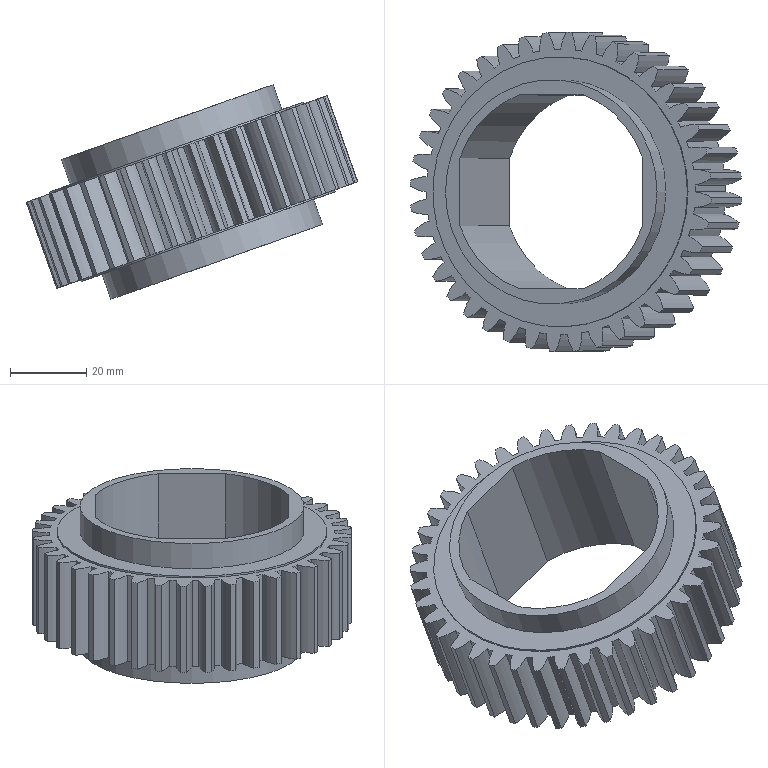Part | STEP file | GEAR1-1_id514_x_t | 1 solid | 178 faces | box 87.142 x 83.945 x 56.458 mm | volume 75327 mm3 | cylinder 168 | plane 10 | commonest cylinder face diameters 23.751 x80 75 x40 84 x40 54 x4 59 x2 71 x2